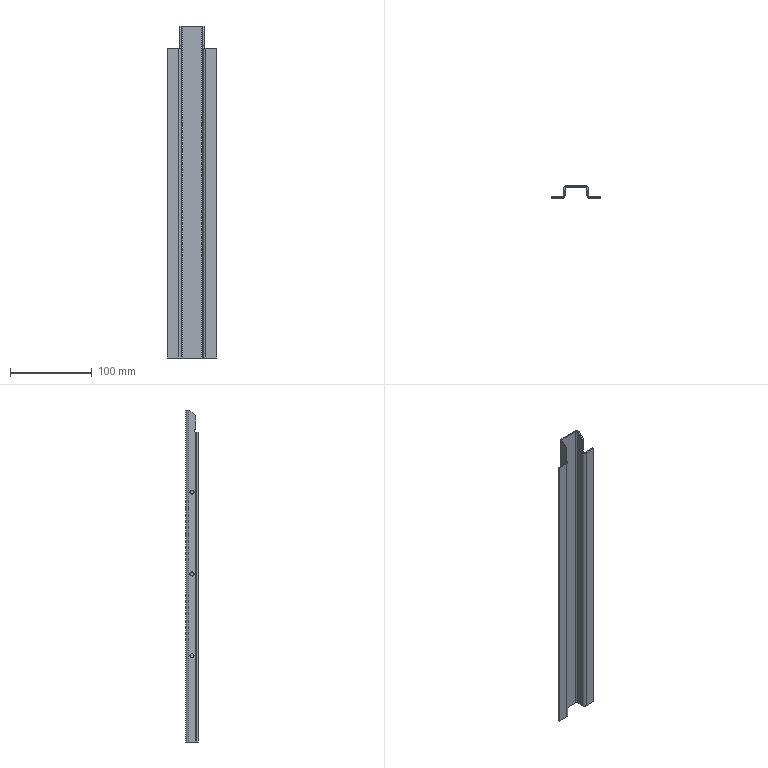Part | SolidWorks | features ICE 2, Chamfer 1, Fillet 1, FlatPattern 1, SMBaseFlange 1, SheetMetal 1 | 1 solid | 58 faces | box 60 x 15 x 406 mm | volume 52147 mm3 | plane 40 | cylinder 18 | commonest cylinder face diameters 3 x8 5 x6 6.2 x4